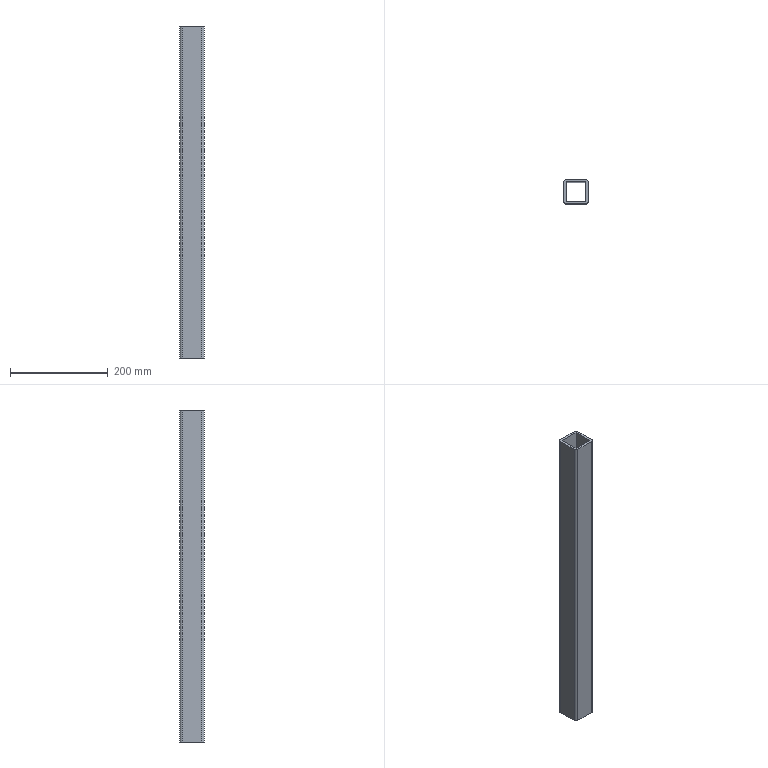Part | STEP file | SOLID | 1 solid | 14 faces | box 50 x 50 x 680 mm | volume 597407 mm3 | plane 10 | cylinder 4 | commonest cylinder face diameters 10 x4
STEP:
#1=CARTESIAN_POINT('',(0.,0.,0.));
#2=DIRECTION('',(0.,0.,1.));
#3=DIRECTION('',(1.,0.,0.));
#4=AXIS2_PLACEMENT_3D('',#1,#2,#3);
#5=CARTESIAN_POINT('',(-758.5,-310.,-70.));
#6=VERTEX_POINT('',#5);
#7=CARTESIAN_POINT('',(-758.5,-270.,-70.));
#8=VERTEX_POINT('',#7);
#9=CARTESIAN_POINT('',(-758.5,-310.,-70.));
#10=DIRECTION('',(0.,1.,0.));
#11=VECTOR('',#10,1.);
#12=LINE('',#9,#11);
#13=CARTESIAN_POINT('',(-758.5,-310.,-670.));
#14=DIRECTION('',(1.,0.,0.));
#15=DIRECTION('',(0.,1.,0.));
#16=AXIS2_PLACEMENT_3D('',#13,#14,#15);
#17=PLANE('',#16);
#18=CARTESIAN_POINT('',(0.,600.));
#19=DIRECTION('',(1.,0.));
#20=VECTOR('',#19,1.);
#21=LINE('',#18,#20);
#22=(GEOMETRIC_REPRESENTATION_CONTEXT(2)PARAMETRIC_REPRESENTATION_CONTEXT()REPRESENTATION_CONTEXT('',''));
#23=DEFINITIONAL_REPRESENTATION('',(#21),#22);
#24=PCURVE('',#17,#23);
#25=CARTESIAN_POINT('',(826.5,-310.,-70.));
#26=DIRECTION('',(0.,0.,1.));
#27=DIRECTION('',(0.,-1.,0.));
#28=AXIS2_PLACEMENT_3D('',#25,#26,#27);
#29=PLANE('',#28);
#30=CARTESIAN_POINT('',(0.,-1585.));
#31=DIRECTION('',(-1.,0.));
#32=VECTOR('',#31,1.);
#33=LINE('',#30,#32);
#34=(GEOMETRIC_REPRESENTATION_CONTEXT(2)PARAMETRIC_REPRESENTATION_CONTEXT()REPRESENTATION_CONTEXT('',''));
#35=DEFINITIONAL_REPRESENTATION('',(#33),#34);
#36=PCURVE('',#29,#35);
#37=SURFACE_CURVE('',#12,(#24,#36),.PCURVE_S1.);
#38=EDGE_CURVE('',#6,#8,#37,.T.);
#39=ORIENTED_EDGE('',*,*,#38,.T.);
#40=CARTESIAN_POINT('',(-758.5,-270.,-750.));
#41=VERTEX_POINT('',#40);
#42=CARTESIAN_POINT('',(-758.5,-270.,-670.));
#43=DIRECTION('',(0.,0.,1.));
#44=VECTOR('',#43,1.);
#45=LINE('',#42,#44);
#46=CARTESIAN_POINT('',(40.,0.));
#47=DIRECTION('',(0.,1.));
#48=VECTOR('',#47,1.);
#49=LINE('',#46,#48);
#50=(GEOMETRIC_REPRESENTATION_CONTEXT(2)PARAMETRIC_REPRESENTATION_CONTEXT()REPRESENTATION_CONTEXT('',''));
#51=DEFINITIONAL_REPRESENTATION('',(#49),#50);
#52=PCURVE('',#17,#51);
#53=CARTESIAN_POINT('',(-758.5,-270.,-670.));
#54=DIRECTION('',(0.,1.,0.));
#55=DIRECTION('',(-1.,0.,0.));
#56=AXIS2_PLACEMENT_3D('',#53,#54,#55);
#57=PLANE('',#56);
#58=CARTESIAN_POINT('',(0.,0.));
#59=DIRECTION('',(0.,1.));
#60=VECTOR('',#59,1.);
#61=LINE('',#58,#60);
#62=(GEOMETRIC_REPRESENTATION_CONTEXT(2)PARAMETRIC_REPRESENTATION_CONTEXT()REPRESENTATION_CONTEXT('',''));
#63=DEFINITIONAL_REPRESENTATION('',(#61),#62);
#64=PCURVE('',#57,#63);
#65=SURFACE_CURVE('',#45,(#52,#64),.PCURVE_S1.);
#66=EDGE_CURVE('',#41,#8,#65,.T.);
#67=ORIENTED_EDGE('',*,*,#66,.F.);
#68=CARTESIAN_POINT('',(-758.5,-310.,-750.));
#69=VERTEX_POINT('',#68);
#70=CARTESIAN_POINT('',(-758.5,-310.,-750.));
#71=DIRECTION('',(0.,1.,0.));
#72=VECTOR('',#71,1.);
#73=LINE('',#70,#72);
#74=CARTESIAN_POINT('',(0.,-80.));
#75=DIRECTION('',(1.,0.));
#76=VECTOR('',#75,1.);
#77=LINE('',#74,#76);
#78=(GEOMETRIC_REPRESENTATION_CONTEXT(2)PARAMETRIC_REPRESENTATION_CONTEXT()REPRESENTATION_CONTEXT('',''));
#79=DEFINITIONAL_REPRESENTATION('',(#77),#78);
#80=PCURVE('',#17,#79);
#81=CARTESIAN_POINT('',(796.5,-310.,-750.));
#82=DIRECTION('',(0.,0.,1.));
#83=DIRECTION('',(0.,-1.,0.));
#84=AXIS2_PLACEMENT_3D('',#81,#82,#83);
#85=PLANE('',#84);
#86=CARTESIAN_POINT('',(0.,-1555.));
#87=DIRECTION('',(-1.,0.));
#88=VECTOR('',#87,1.);
#89=LINE('',#86,#88);
#90=(GEOMETRIC_REPRESENTATION_CONTEXT(2)PARAMETRIC_REPRESENTATION_CONTEXT()REPRESENTATION_CONTEXT('',''));
#91=DEFINITIONAL_REPRESENTATION('',(#89),#90);
#92=PCURVE('',#85,#91);
#93=SURFACE_CURVE('',#73,(#80,#92),.PCURVE_S1.);
#94=EDGE_CURVE('',#69,#41,#93,.T.);
#95=ORIENTED_EDGE('',*,*,#94,.F.);
#96=CARTESIAN_POINT('',(-758.5,-310.,-670.));
#97=DIRECTION('',(0.,0.,1.));
#98=VECTOR('',#97,1.);
#99=LINE('',#96,#98);
#100=CARTESIAN_POINT('',(0.,0.));
#101=DIRECTION('',(0.,1.));
#102=VECTOR('',#101,1.);
#103=LINE('',#100,#102);
#104=(GEOMETRIC_REPRESENTATION_CONTEXT(2)PARAMETRIC_REPRESENTATION_CONTEXT()REPRESENTATION_CONTEXT('',''));
#105=DEFINITIONAL_REPRESENTATION('',(#103),#104);
#106=PCURVE('',#17,#105);
#107=CARTESIAN_POINT('',(-798.5,-310.,-670.));
#108=DIRECTION('',(0.,-1.,0.));
#109=DIRECTION('',(0.,0.,1.));
#110=AXIS2_PLACEMENT_3D('',#107,#108,#109);
#111=PLANE('',#110);
#112=CARTESIAN_POINT('',(0.,-40.));
#113=DIRECTION('',(1.,0.));
#114=VECTOR('',#113,1.);
#115=LINE('',#112,#114);
#116=(GEOMETRIC_REPRESENTATION_CONTEXT(2)PARAMETRIC_REPRESENTATION_CONTEXT()REPRESENTATION_CONTEXT('',''));
#117=DEFINITIONAL_REPRESENTATION('',(#115),#116);
#118=PCURVE('',#111,#117);
#119=SURFACE_CURVE('',#99,(#106,#118),.PCURVE_S1.);
#120=EDGE_CURVE('',#69,#6,#119,.T.);
#121=ORIENTED_EDGE('',*,*,#120,.T.);
#122=EDGE_LOOP('',(#39,#67,#95,#121));
#123=FACE_BOUND('',#122,.T.);
#124=ADVANCED_FACE('',(#123),#17,.F.);
#125=CARTESIAN_POINT('',(-798.5,-270.,-70.));
#126=VERTEX_POINT('',#125);
#127=CARTESIAN_POINT('',(-758.5,-270.,-70.));
#128=DIRECTION('',(-1.,0.,0.));
#129=VECTOR('',#128,1.);
#130=LINE('',#127,#129);
#131=CARTESIAN_POINT('',(0.,600.));
#132=DIRECTION('',(1.,0.));
#133=VECTOR('',#132,1.);
#134=LINE('',#131,#133);
#135=(GEOMETRIC_REPRESENTATION_CONTEXT(2)PARAMETRIC_REPRESENTATION_CONTEXT()REPRESENTATION_CONTEXT('',''));
#136=DEFINITIONAL_REPRESENTATION('',(#134),#135);
#137=PCURVE('',#57,#136);
#138=CARTESIAN_POINT('',(-40.,-1585.));
#139=DIRECTION('',(0.,-1.));
#140=VECTOR('',#139,1.);
#141=LINE('',#138,#140);
#142=(GEOMETRIC_REPRESENTATION_CONTEXT(2)PARAMETRIC_REPRESENTATION_CONTEXT()REPRESENTATION_CONTEXT('',''));
#143=DEFINITIONAL_REPRESENTATION('',(#141),#142);
#144=PCURVE('',#29,#143);
#145=SURFACE_CURVE('',#130,(#137,#144),.PCURVE_S1.);
#146=EDGE_CURVE('',#8,#126,#145,.T.);
#147=ORIENTED_EDGE('',*,*,#146,.T.);
#148=CARTESIAN_POINT('',(-798.5,-270.,-750.));
#149=VERTEX_POINT('',#148);
#150=CARTESIAN_POINT('',(-798.5,-270.,-670.));
#151=DIRECTION('',(0.,0.,1.));
#152=VECTOR('',#151,1.);
#153=LINE('',#150,#152);
#154=CARTESIAN_POINT('',(40.,0.));
#155=DIRECTION('',(0.,1.));
#156=VECTOR('',#155,1.);
#157=LINE('',#154,#156);
#158=(GEOMETRIC_REPRESENTATION_CONTEXT(2)PARAMETRIC_REPRESENTATION_CONTEXT()REPRESENTATION_CONTEXT('',''));
#159=DEFINITIONAL_REPRESENTATION('',(#157),#158);
#160=PCURVE('',#57,#159);
#161=CARTESIAN_POINT('',(-798.5,-270.,-670.));
#162=DIRECTION('',(-1.,0.,0.));
#163=DIRECTION('',(0.,0.,-1.));
#164=AXIS2_PLACEMENT_3D('',#161,#162,#163);
#165=PLANE('',#164);
#166=CARTESIAN_POINT('',(0.,0.));
#167=DIRECTION('',(-1.,0.));
#168=VECTOR('',#167,1.);
#169=LINE('',#166,#168);
#170=(GEOMETRIC_REPRESENTATION_CONTEXT(2)PARAMETRIC_REPRESENTATION_CONTEXT()REPRESENTATION_CONTEXT('',''));
#171=DEFINITIONAL_REPRESENTATION('',(#169),#170);
#172=PCURVE('',#165,#171);
#173=SURFACE_CURVE('',#153,(#160,#172),.PCURVE_S1.);
#174=EDGE_CURVE('',#149,#126,#173,.T.);
#175=ORIENTED_EDGE('',*,*,#174,.F.);
#176=CARTESIAN_POINT('',(-758.5,-270.,-750.));
#177=DIRECTION('',(-1.,0.,0.));
#178=VECTOR('',#177,1.);
#179=LINE('',#176,#178);
#180=CARTESIAN_POINT('',(0.,-80.));
#181=DIRECTION('',(1.,0.));
#182=VECTOR('',#181,1.);
#183=LINE('',#180,#182);
#184=(GEOMETRIC_REPRESENTATION_CONTEXT(2)PARAMETRIC_REPRESENTATION_CONTEXT()REPRESENTATION_CONTEXT('',''));
#185=DEFINITIONAL_REPRESENTATION('',(#183),#184);
#186=PCURVE('',#57,#185);
#187=CARTESIAN_POINT('',(-40.,-1555.));
#188=DIRECTION('',(0.,-1.));
#189=VECTOR('',#188,1.);
#190=LINE('',#187,#189);
#191=(GEOMETRIC_REPRESENTATION_CONTEXT(2)PARAMETRIC_REPRESENTATION_CONTEXT()REPRESENTATION_CONTEXT('',''));
#192=DEFINITIONAL_REPRESENTATION('',(#190),#191);
#193=PCURVE('',#85,#192);
#194=SURFACE_CURVE('',#179,(#186,#193),.PCURVE_S1.);
#195=EDGE_CURVE('',#41,#149,#194,.T.);
#196=ORIENTED_EDGE('',*,*,#195,.F.);
#197=ORIENTED_EDGE('',*,*,#66,.T.);
#198=EDGE_LOOP('',(#147,#175,#196,#197));
#199=FACE_BOUND('',#198,.T.);
#200=ADVANCED_FACE('',(#199),#57,.F.);
#201=CARTESIAN_POINT('',(-798.5,-310.,-70.));
#202=VERTEX_POINT('',#201);
#203=CARTESIAN_POINT('',(-798.5,-270.,-70.));
#204=DIRECTION('',(0.,-1.,0.));
#205=VECTOR('',#204,1.);
#206=LINE('',#203,#205);
#207=CARTESIAN_POINT('',(-600.,0.));
#208=DIRECTION('',(0.,1.));
#209=VECTOR('',#208,1.);
#210=LINE('',#207,#209);
#211=(GEOMETRIC_REPRESENTATION_CONTEXT(2)PARAMETRIC_REPRESENTATION_CONTEXT()REPRESENTATION_CONTEXT('',''));
#212=DEFINITIONAL_REPRESENTATION('',(#210),#211);
#213=PCURVE('',#165,#212);
#214=CARTESIAN_POINT('',(-40.,-1625.));
#215=DIRECTION('',(1.,0.));
#216=VECTOR('',#215,1.);
#217=LINE('',#214,#216);
#218=(GEOMETRIC_REPRESENTATION_CONTEXT(2)PARAMETRIC_REPRESENTATION_CONTEXT()REPRESENTATION_CONTEXT('',''));
#219=DEFINITIONAL_REPRESENTATION('',(#217),#218);
#220=PCURVE('',#29,#219);
#221=SURFACE_CURVE('',#206,(#213,#220),.PCURVE_S1.);
#222=EDGE_CURVE('',#126,#202,#221,.T.);
#223=ORIENTED_EDGE('',*,*,#222,.T.);
#224=CARTESIAN_POINT('',(-798.5,-310.,-750.));
#225=VERTEX_POINT('',#224);
#226=CARTESIAN_POINT('',(-798.5,-310.,-670.));
#227=DIRECTION('',(0.,0.,1.));
#228=VECTOR('',#227,1.);
#229=LINE('',#226,#228);
#230=CARTESIAN_POINT('',(0.,40.));
#231=DIRECTION('',(-1.,0.));
#232=VECTOR('',#231,1.);
#233=LINE('',#230,#232);
#234=(GEOMETRIC_REPRESENTATION_CONTEXT(2)PARAMETRIC_REPRESENTATION_CONTEXT()REPRESENTATION_CONTEXT('',''));
#235=DEFINITIONAL_REPRESENTATION('',(#233),#234);
#236=PCURVE('',#165,#235);
#237=CARTESIAN_POINT('',(0.,0.));
#238=DIRECTION('',(1.,0.));
#239=VECTOR('',#238,1.);
#240=LINE('',#237,#239);
#241=(GEOMETRIC_REPRESENTATION_CONTEXT(2)PARAMETRIC_REPRESENTATION_CONTEXT()REPRESENTATION_CONTEXT('',''));
#242=DEFINITIONAL_REPRESENTATION('',(#240),#241);
#243=PCURVE('',#111,#242);
#244=SURFACE_CURVE('',#229,(#236,#243),.PCURVE_S1.);
#245=EDGE_CURVE('',#225,#202,#244,.T.);
#246=ORIENTED_EDGE('',*,*,#245,.F.);
#247=CARTESIAN_POINT('',(-798.5,-270.,-750.));
#248=DIRECTION('',(0.,-1.,0.));
#249=VECTOR('',#248,1.);
#250=LINE('',#247,#249);
#251=CARTESIAN_POINT('',(80.,0.));
#252=DIRECTION('',(0.,1.));
#253=VECTOR('',#252,1.);
#254=LINE('',#251,#253);
#255=(GEOMETRIC_REPRESENTATION_CONTEXT(2)PARAMETRIC_REPRESENTATION_CONTEXT()REPRESENTATION_CONTEXT('',''));
#256=DEFINITIONAL_REPRESENTATION('',(#254),#255);
#257=PCURVE('',#165,#256);
#258=CARTESIAN_POINT('',(-40.,-1595.));
#259=DIRECTION('',(1.,0.));
#260=VECTOR('',#259,1.);
#261=LINE('',#258,#260);
#262=(GEOMETRIC_REPRESENTATION_CONTEXT(2)PARAMETRIC_REPRESENTATION_CONTEXT()REPRESENTATION_CONTEXT('',''));
#263=DEFINITIONAL_REPRESENTATION('',(#261),#262);
#264=PCURVE('',#85,#263);
#265=SURFACE_CURVE('',#250,(#257,#264),.PCURVE_S1.);
#266=EDGE_CURVE('',#149,#225,#265,.T.);
#267=ORIENTED_EDGE('',*,*,#266,.F.);
#268=ORIENTED_EDGE('',*,*,#174,.T.);
#269=EDGE_LOOP('',(#223,#246,#267,#268));
#270=FACE_BOUND('',#269,.T.);
#271=ADVANCED_FACE('',(#270),#165,.F.);
#272=CARTESIAN_POINT('',(-753.5,-270.,-70.));
#273=VERTEX_POINT('',#272);
#274=CARTESIAN_POINT('',(-753.5,-310.,-70.));
#275=VERTEX_POINT('',#274);
#276=CARTESIAN_POINT('',(-753.5,-270.,-70.));
#277=DIRECTION('',(0.,-1.,0.));
#278=VECTOR('',#277,1.);
#279=LINE('',#276,#278);
#280=CARTESIAN_POINT('',(-753.5,-270.,-670.));
#281=DIRECTION('',(-1.,0.,0.));
#282=DIRECTION('',(0.,-1.,0.));
#283=AXIS2_PLACEMENT_3D('',#280,#281,#282);
#284=PLANE('',#283);
#285=CARTESIAN_POINT('',(0.,600.));
#286=DIRECTION('',(1.,0.));
#287=VECTOR('',#286,1.);
#288=LINE('',#285,#287);
#289=(GEOMETRIC_REPRESENTATION_CONTEXT(2)PARAMETRIC_REPRESENTATION_CONTEXT()REPRESENTATION_CONTEXT('',''));
#290=DEFINITIONAL_REPRESENTATION('',(#288),#289);
#291=PCURVE('',#284,#290);
#292=CARTESIAN_POINT('',(-40.,-1580.));
#293=DIRECTION('',(1.,0.));
#294=VECTOR('',#293,1.);
#295=LINE('',#292,#294);
#296=(GEOMETRIC_REPRESENTATION_CONTEXT(2)PARAMETRIC_REPRESENTATION_CONTEXT()REPRESENTATION_CONTEXT('',''));
#297=DEFINITIONAL_REPRESENTATION('',(#295),#296);
#298=PCURVE('',#29,#297);
#299=SURFACE_CURVE('',#279,(#291,#298),.PCURVE_S1.);
#300=EDGE_CURVE('',#273,#275,#299,.T.);
#301=ORIENTED_EDGE('',*,*,#300,.T.);
#302=CARTESIAN_POINT('',(-753.5,-310.,-750.));
#303=VERTEX_POINT('',#302);
#304=CARTESIAN_POINT('',(-753.5,-310.,-670.));
#305=DIRECTION('',(0.,0.,1.));
#306=VECTOR('',#305,1.);
#307=LINE('',#304,#306);
#308=CARTESIAN_POINT('',(40.,0.));
#309=DIRECTION('',(0.,1.));
#310=VECTOR('',#309,1.);
#311=LINE('',#308,#310);
#312=(GEOMETRIC_REPRESENTATION_CONTEXT(2)PARAMETRIC_REPRESENTATION_CONTEXT()REPRESENTATION_CONTEXT('',''));
#313=DEFINITIONAL_REPRESENTATION('',(#311),#312);
#314=PCURVE('',#284,#313);
#315=CARTESIAN_POINT('',(-758.5,-310.,-670.));
#316=DIRECTION('',(0.,0.,1.));
#317=DIRECTION('',(0.,1.,0.));
#318=AXIS2_PLACEMENT_3D('',#315,#316,#317);
#319=CYLINDRICAL_SURFACE('',#318,5.);
#320=CARTESIAN_POINT('',(4.712,0.));
#321=DIRECTION('',(0.,1.));
#322=VECTOR('',#321,1.);
#323=LINE('',#320,#322);
#324=(GEOMETRIC_REPRESENTATION_CONTEXT(2)PARAMETRIC_REPRESENTATION_CONTEXT()REPRESENTATION_CONTEXT('',''));
#325=DEFINITIONAL_REPRESENTATION('',(#323),#324);
#326=PCURVE('',#319,#325);
#327=SURFACE_CURVE('',#307,(#314,#326),.PCURVE_S1.);
#328=EDGE_CURVE('',#303,#275,#327,.T.);
#329=ORIENTED_EDGE('',*,*,#328,.F.);
#330=CARTESIAN_POINT('',(-753.5,-270.,-750.));
#331=VERTEX_POINT('',#330);
#332=CARTESIAN_POINT('',(-753.5,-270.,-750.));
#333=DIRECTION('',(0.,-1.,0.));
#334=VECTOR('',#333,1.);
#335=LINE('',#332,#334);
#336=CARTESIAN_POINT('',(0.,-80.));
#337=DIRECTION('',(1.,0.));
#338=VECTOR('',#337,1.);
#339=LINE('',#336,#338);
#340=(GEOMETRIC_REPRESENTATION_CONTEXT(2)PARAMETRIC_REPRESENTATION_CONTEXT()REPRESENTATION_CONTEXT('',''));
#341=DEFINITIONAL_REPRESENTATION('',(#339),#340);
#342=PCURVE('',#284,#341);
#343=CARTESIAN_POINT('',(-40.,-1550.));
#344=DIRECTION('',(1.,0.));
#345=VECTOR('',#344,1.);
#346=LINE('',#343,#345);
#347=(GEOMETRIC_REPRESENTATION_CONTEXT(2)PARAMETRIC_REPRESENTATION_CONTEXT()REPRESENTATION_CONTEXT('',''));
#348=DEFINITIONAL_REPRESENTATION('',(#346),#347);
#349=PCURVE('',#85,#348);
#350=SURFACE_CURVE('',#335,(#342,#349),.PCURVE_S1.);
#351=EDGE_CURVE('',#331,#303,#350,.T.);
#352=ORIENTED_EDGE('',*,*,#351,.F.);
#353=CARTESIAN_POINT('',(-753.5,-270.,-670.));
#354=DIRECTION('',(0.,0.,1.));
#355=VECTOR('',#354,1.);
#356=LINE('',#353,#355);
#357=CARTESIAN_POINT('',(0.,0.));
#358=DIRECTION('',(0.,1.));
#359=VECTOR('',#358,1.);
#360=LINE('',#357,#359);
#361=(GEOMETRIC_REPRESENTATION_CONTEXT(2)PARAMETRIC_REPRESENTATION_CONTEXT()REPRESENTATION_CONTEXT('',''));
#362=DEFINITIONAL_REPRESENTATION('',(#360),#361);
#363=PCURVE('',#284,#362);
#364=CARTESIAN_POINT('',(-758.5,-270.,-670.));
#365=DIRECTION('',(0.,0.,1.));
#366=DIRECTION('',(0.,1.,0.));
#367=AXIS2_PLACEMENT_3D('',#364,#365,#366);
#368=CYLINDRICAL_SURFACE('',#367,5.);
#369=CARTESIAN_POINT('',(4.712,0.));
#370=DIRECTION('',(0.,1.));
#371=VECTOR('',#370,1.);
#372=LINE('',#369,#371);
#373=(GEOMETRIC_REPRESENTATION_CONTEXT(2)PARAMETRIC_REPRESENTATION_CONTEXT()REPRESENTATION_CONTEXT('',''));
#374=DEFINITIONAL_REPRESENTATION('',(#372),#373);
#375=PCURVE('',#368,#374);
#376=SURFACE_CURVE('',#356,(#363,#375),.PCURVE_S1.);
#377=EDGE_CURVE('',#331,#273,#376,.T.);
#378=ORIENTED_EDGE('',*,*,#377,.T.);
#379=EDGE_LOOP('',(#301,#329,#352,#378));
#380=FACE_BOUND('',#379,.T.);
#381=ADVANCED_FACE('',(#380),#284,.F.);
#382=CARTESIAN_POINT('',(-758.5,-315.,-70.));
#383=VERTEX_POINT('',#382);
#384=CARTESIAN_POINT('',(-758.5,-310.,-70.));
#385=DIRECTION('',(0.,0.,-1.));
#386=DIRECTION('',(0.,1.,0.));
#387=AXIS2_PLACEMENT_3D('',#384,#385,#386);
#388=CIRCLE('',#387,5.);
#389=CARTESIAN_POINT('',(6.283,600.));
#390=DIRECTION('',(-1.,0.));
#391=VECTOR('',#390,1.);
#392=LINE('',#389,#391);
#393=(GEOMETRIC_REPRESENTATION_CONTEXT(2)PARAMETRIC_REPRESENTATION_CONTEXT()REPRESENTATION_CONTEXT('',''));
#394=DEFINITIONAL_REPRESENTATION('',(#392),#393);
#395=PCURVE('',#319,#394);
#396=CARTESIAN_POINT('',(-5.,-1585.));
#397=CARTESIAN_POINT('',(-5.,-1576.34));
#398=CARTESIAN_POINT('',(2.5,-1580.67));
#399=CARTESIAN_POINT('',(10.,-1585.));
#400=CARTESIAN_POINT('',(2.5,-1589.33));
#401=CARTESIAN_POINT('',(-5.,-1593.66));
#402=CARTESIAN_POINT('',(-5.,-1585.));
#403=(BOUNDED_CURVE()B_SPLINE_CURVE(2,(#396,#397,#398,#399,#400,#401,#402),.UNSPECIFIED.,.T.,.F.)B_SPLINE_CURVE_WITH_KNOTS((1,2,2,2,2,1),(-2.094,0.,2.094,4.189,6.283,8.378),.UNSPECIFIED.)CURVE()GEOMETRIC_REPRESENTATION_ITEM()RATIONAL_B_SPLINE_CURVE((1.,0.5,1.,0.5,1.,0.5,1.))REPRESENTATION_ITEM(''));
#404=(GEOMETRIC_REPRESENTATION_CONTEXT(2)PARAMETRIC_REPRESENTATION_CONTEXT()REPRESENTATION_CONTEXT('',''));
#405=DEFINITIONAL_REPRESENTATION('',(#403),#404);
#406=PCURVE('',#29,#405);
#407=SURFACE_CURVE('',#388,(#395,#406),.PCURVE_S1.);
#408=EDGE_CURVE('',#275,#383,#407,.T.);
#409=ORIENTED_EDGE('',*,*,#408,.T.);
#410=CARTESIAN_POINT('',(-758.5,-315.,-750.));
#411=VERTEX_POINT('',#410);
#412=CARTESIAN_POINT('',(-758.5,-315.,-670.));
#413=DIRECTION('',(0.,0.,1.));
#414=VECTOR('',#413,1.);
#415=LINE('',#412,#414);
#416=CARTESIAN_POINT('',(3.142,0.));
#417=DIRECTION('',(0.,1.));
#418=VECTOR('',#417,1.);
#419=LINE('',#416,#418);
#420=(GEOMETRIC_REPRESENTATION_CONTEXT(2)PARAMETRIC_REPRESENTATION_CONTEXT()REPRESENTATION_CONTEXT('',''));
#421=DEFINITIONAL_REPRESENTATION('',(#419),#420);
#422=PCURVE('',#319,#421);
#423=CARTESIAN_POINT('',(-758.5,-315.,-670.));
#424=DIRECTION('',(0.,1.,0.));
#425=DIRECTION('',(0.,0.,-1.));
#426=AXIS2_PLACEMENT_3D('',#423,#424,#425);
#427=PLANE('',#426);
#428=CARTESIAN_POINT('',(0.,0.));
#429=DIRECTION('',(-1.,0.));
#430=VECTOR('',#429,1.);
#431=LINE('',#428,#430);
#432=(GEOMETRIC_REPRESENTATION_CONTEXT(2)PARAMETRIC_REPRESENTATION_CONTEXT()REPRESENTATION_CONTEXT('',''));
#433=DEFINITIONAL_REPRESENTATION('',(#431),#432);
#434=PCURVE('',#427,#433);
#435=SURFACE_CURVE('',#415,(#422,#434),.PCURVE_S1.);
#436=EDGE_CURVE('',#411,#383,#435,.T.);
#437=ORIENTED_EDGE('',*,*,#436,.F.);
#438=CARTESIAN_POINT('',(-758.5,-310.,-750.));
#439=DIRECTION('',(0.,0.,-1.));
#440=DIRECTION('',(0.,-1.,0.));
#441=AXIS2_PLACEMENT_3D('',#438,#439,#440);
#442=CIRCLE('',#441,5.);
#443=CARTESIAN_POINT('',(9.425,-80.));
#444=DIRECTION('',(-1.,0.));
#445=VECTOR('',#444,1.);
#446=LINE('',#443,#445);
#447=(GEOMETRIC_REPRESENTATION_CONTEXT(2)PARAMETRIC_REPRESENTATION_CONTEXT()REPRESENTATION_CONTEXT('',''));
#448=DEFINITIONAL_REPRESENTATION('',(#446),#447);
#449=PCURVE('',#319,#448);
#450=CARTESIAN_POINT('',(5.,-1555.));
#451=CARTESIAN_POINT('',(5.,-1563.66));
#452=CARTESIAN_POINT('',(-2.5,-1559.33));
#453=CARTESIAN_POINT('',(-10.,-1555.));
#454=CARTESIAN_POINT('',(-2.5,-1550.67));
#455=CARTESIAN_POINT('',(5.,-1546.34));
#456=CARTESIAN_POINT('',(5.,-1555.));
#457=(BOUNDED_CURVE()B_SPLINE_CURVE(2,(#450,#451,#452,#453,#454,#455,#456),.UNSPECIFIED.,.T.,.F.)B_SPLINE_CURVE_WITH_KNOTS((1,2,2,2,2,1),(-2.094,0.,2.094,4.189,6.283,8.378),.UNSPECIFIED.)CURVE()GEOMETRIC_REPRESENTATION_ITEM()RATIONAL_B_SPLINE_CURVE((1.,0.5,1.,0.5,1.,0.5,1.))REPRESENTATION_ITEM(''));
#458=(GEOMETRIC_REPRESENTATION_CONTEXT(2)PARAMETRIC_REPRESENTATION_CONTEXT()REPRESENTATION_CONTEXT('',''));
#459=DEFINITIONAL_REPRESENTATION('',(#457),#458);
#460=PCURVE('',#85,#459);
#461=SURFACE_CURVE('',#442,(#449,#460),.PCURVE_S1.);
#462=EDGE_CURVE('',#303,#411,#461,.T.);
#463=ORIENTED_EDGE('',*,*,#462,.F.);
#464=ORIENTED_EDGE('',*,*,#328,.T.);
#465=EDGE_LOOP('',(#409,#437,#463,#464));
#466=FACE_BOUND('',#465,.T.);
#467=ADVANCED_FACE('',(#466),#319,.T.);
#468=CARTESIAN_POINT('',(-798.5,-315.,-70.));
#469=VERTEX_POINT('',#468);
#470=CARTESIAN_POINT('',(-758.5,-315.,-70.));
#471=DIRECTION('',(-1.,0.,0.));
#472=VECTOR('',#471,1.);
#473=LINE('',#470,#472);
#474=CARTESIAN_POINT('',(-600.,0.));
#475=DIRECTION('',(0.,1.));
#476=VECTOR('',#475,1.);
#477=LINE('',#474,#476);
#478=(GEOMETRIC_REPRESENTATION_CONTEXT(2)PARAMETRIC_REPRESENTATION_CONTEXT()REPRESENTATION_CONTEXT('',''));
#479=DEFINITIONAL_REPRESENTATION('',(#477),#478);
#480=PCURVE('',#427,#479);
#481=CARTESIAN_POINT('',(5.,-1585.));
#482=DIRECTION('',(0.,-1.));
#483=VECTOR('',#482,1.);
#484=LINE('',#481,#483);
#485=(GEOMETRIC_REPRESENTATION_CONTEXT(2)PARAMETRIC_REPRESENTATION_CONTEXT()REPRESENTATION_CONTEXT('',''));
#486=DEFINITIONAL_REPRESENTATION('',(#484),#485);
#487=PCURVE('',#29,#486);
#488=SURFACE_CURVE('',#473,(#480,#487),.PCURVE_S1.);
#489=EDGE_CURVE('',#383,#469,#488,.T.);
#490=ORIENTED_EDGE('',*,*,#489,.T.);
#491=CARTESIAN_POINT('',(-798.5,-315.,-750.));
#492=VERTEX_POINT('',#491);
#493=CARTESIAN_POINT('',(-798.5,-315.,-670.));
#494=DIRECTION('',(0.,0.,1.));
#495=VECTOR('',#494,1.);
#496=LINE('',#493,#495);
#497=CARTESIAN_POINT('',(0.,40.));
#498=DIRECTION('',(-1.,0.));
#499=VECTOR('',#498,1.);
#500=LINE('',#497,#499);
#501=(GEOMETRIC_REPRESENTATION_CONTEXT(2)PARAMETRIC_REPRESENTATION_CONTEXT()REPRESENTATION_CONTEXT('',''));
#502=DEFINITIONAL_REPRESENTATION('',(#500),#501);
#503=PCURVE('',#427,#502);
#504=CARTESIAN_POINT('',(-798.5,-310.,-670.));
#505=DIRECTION('',(0.,0.,1.));
#506=DIRECTION('',(0.,1.,0.));
#507=AXIS2_PLACEMENT_3D('',#504,#505,#506);
#508=CYLINDRICAL_SURFACE('',#507,5.);
#509=CARTESIAN_POINT('',(3.142,0.));
#510=DIRECTION('',(0.,1.));
#511=VECTOR('',#510,1.);
#512=LINE('',#509,#511);
#513=(GEOMETRIC_REPRESENTATION_CONTEXT(2)PARAMETRIC_REPRESENTATION_CONTEXT()REPRESENTATION_CONTEXT('',''));
#514=DEFINITIONAL_REPRESENTATION('',(#512),#513);
#515=PCURVE('',#508,#514);
#516=SURFACE_CURVE('',#496,(#503,#515),.PCURVE_S1.);
#517=EDGE_CURVE('',#492,#469,#516,.T.);
#518=ORIENTED_EDGE('',*,*,#517,.F.);
#519=CARTESIAN_POINT('',(-758.5,-315.,-750.));
#520=DIRECTION('',(-1.,0.,0.));
#521=VECTOR('',#520,1.);
#522=LINE('',#519,#521);
#523=CARTESIAN_POINT('',(80.,0.));
#524=DIRECTION('',(0.,1.));
#525=VECTOR('',#524,1.);
#526=LINE('',#523,#525);
#527=(GEOMETRIC_REPRESENTATION_CONTEXT(2)PARAMETRIC_REPRESENTATION_CONTEXT()REPRESENTATION_CONTEXT('',''));
#528=DEFINITIONAL_REPRESENTATION('',(#526),#527);
#529=PCURVE('',#427,#528);
#530=CARTESIAN_POINT('',(5.,-1555.));
#531=DIRECTION('',(0.,-1.));
#532=VECTOR('',#531,1.);
#533=LINE('',#530,#532);
#534=(GEOMETRIC_REPRESENTATION_CONTEXT(2)PARAMETRIC_REPRESENTATION_CONTEXT()REPRESENTATION_CONTEXT('',''));
#535=DEFINITIONAL_REPRESENTATION('',(#533),#534);
#536=PCURVE('',#85,#535);
#537=SURFACE_CURVE('',#522,(#529,#536),.PCURVE_S1.);
#538=EDGE_CURVE('',#411,#492,#537,.T.);
#539=ORIENTED_EDGE('',*,*,#538,.F.);
#540=ORIENTED_EDGE('',*,*,#436,.T.);
#541=EDGE_LOOP('',(#490,#518,#539,#540));
#542=FACE_BOUND('',#541,.T.);
#543=ADVANCED_FACE('',(#542),#427,.F.);
#544=CARTESIAN_POINT('',(-803.5,-310.,-70.));
#545=VERTEX_POINT('',#544);
#546=CARTESIAN_POINT('',(-798.5,-310.,-70.));
#547=DIRECTION('',(0.,0.,-1.));
#548=DIRECTION('',(0.,1.,0.));
#549=AXIS2_PLACEMENT_3D('',#546,#547,#548);
#550=CIRCLE('',#549,5.);
#551=CARTESIAN_POINT('',(6.283,600.));
#552=DIRECTION('',(-1.,0.));
#553=VECTOR('',#552,1.);
#554=LINE('',#551,#553);
#555=(GEOMETRIC_REPRESENTATION_CONTEXT(2)PARAMETRIC_REPRESENTATION_CONTEXT()REPRESENTATION_CONTEXT('',''));
#556=DEFINITIONAL_REPRESENTATION('',(#554),#555);
#557=PCURVE('',#508,#556);
#558=CARTESIAN_POINT('',(-5.,-1625.));
#559=CARTESIAN_POINT('',(-5.,-1616.34));
#560=CARTESIAN_POINT('',(2.5,-1620.67));
#561=CARTESIAN_POINT('',(10.,-1625.));
#562=CARTESIAN_POINT('',(2.5,-1629.33));
#563=CARTESIAN_POINT('',(-5.,-1633.66));
#564=CARTESIAN_POINT('',(-5.,-1625.));
#565=(BOUNDED_CURVE()B_SPLINE_CURVE(2,(#558,#559,#560,#561,#562,#563,#564),.UNSPECIFIED.,.T.,.F.)B_SPLINE_CURVE_WITH_KNOTS((1,2,2,2,2,1),(-2.094,0.,2.094,4.189,6.283,8.378),.UNSPECIFIED.)CURVE()GEOMETRIC_REPRESENTATION_ITEM()RATIONAL_B_SPLINE_CURVE((1.,0.5,1.,0.5,1.,0.5,1.))REPRESENTATION_ITEM(''));
#566=(GEOMETRIC_REPRESENTATION_CONTEXT(2)PARAMETRIC_REPRESENTATION_CONTEXT()REPRESENTATION_CONTEXT('',''));
#567=DEFINITIONAL_REPRESENTATION('',(#565),#566);
#568=PCURVE('',#29,#567);
#569=SURFACE_CURVE('',#550,(#557,#568),.PCURVE_S1.);
#570=EDGE_CURVE('',#469,#545,#569,.T.);
#571=ORIENTED_EDGE('',*,*,#570,.T.);
#572=CARTESIAN_POINT('',(-803.5,-310.,-750.));
#573=VERTEX_POINT('',#572);
#574=CARTESIAN_POINT('',(-803.5,-310.,-670.));
#575=DIRECTION('',(0.,0.,1.));
#576=VECTOR('',#575,1.);
#577=LINE('',#574,#576);
#578=CARTESIAN_POINT('',(1.571,0.));
#579=DIRECTION('',(0.,1.));
#580=VECTOR('',#579,1.);
#581=LINE('',#578,#580);
#582=(GEOMETRIC_REPRESENTATION_CONTEXT(2)PARAMETRIC_REPRESENTATION_CONTEXT()REPRESENTATION_CONTEXT('',''));
#583=DEFINITIONAL_REPRESENTATION('',(#581),#582);
#584=PCURVE('',#508,#583);
#585=CARTESIAN_POINT('',(-803.5,-310.,-670.));
#586=DIRECTION('',(1.,0.,0.));
#587=DIRECTION('',(0.,0.,1.));
#588=AXIS2_PLACEMENT_3D('',#585,#586,#587);
#589=PLANE('',#588);
#590=CARTESIAN_POINT('',(0.,0.));
#591=DIRECTION('',(1.,0.));
#592=VECTOR('',#591,1.);
#593=LINE('',#590,#592);
#594=(GEOMETRIC_REPRESENTATION_CONTEXT(2)PARAMETRIC_REPRESENTATION_CONTEXT()REPRESENTATION_CONTEXT('',''));
#595=DEFINITIONAL_REPRESENTATION('',(#593),#594);
#596=PCURVE('',#589,#595);
#597=SURFACE_CURVE('',#577,(#584,#596),.PCURVE_S1.);
#598=EDGE_CURVE('',#573,#545,#597,.T.);
#599=ORIENTED_EDGE('',*,*,#598,.F.);
#600=CARTESIAN_POINT('',(-798.5,-310.,-750.));
#601=DIRECTION('',(0.,0.,-1.));
#602=DIRECTION('',(0.,-1.,0.));
#603=AXIS2_PLACEMENT_3D('',#600,#601,#602);
#604=CIRCLE('',#603,5.);
#605=CARTESIAN_POINT('',(3.142,-80.));
#606=DIRECTION('',(-1.,0.));
#607=VECTOR('',#606,1.);
#608=LINE('',#605,#607);
#609=(GEOMETRIC_REPRESENTATION_CONTEXT(2)PARAMETRIC_REPRESENTATION_CONTEXT()REPRESENTATION_CONTEXT('',''));
#610=DEFINITIONAL_REPRESENTATION('',(#608),#609);
#611=PCURVE('',#508,#610);
#612=CARTESIAN_POINT('',(5.,-1595.));
#613=CARTESIAN_POINT('',(5.,-1603.66));
#614=CARTESIAN_POINT('',(-2.5,-1599.33));
#615=CARTESIAN_POINT('',(-10.,-1595.));
#616=CARTESIAN_POINT('',(-2.5,-1590.67));
#617=CARTESIAN_POINT('',(5.,-1586.34));
#618=CARTESIAN_POINT('',(5.,-1595.));
#619=(BOUNDED_CURVE()B_SPLINE_CURVE(2,(#612,#613,#614,#615,#616,#617,#618),.UNSPECIFIED.,.T.,.F.)B_SPLINE_CURVE_WITH_KNOTS((1,2,2,2,2,1),(-2.094,0.,2.094,4.189,6.283,8.378),.UNSPECIFIED.)CURVE()GEOMETRIC_REPRESENTATION_ITEM()RATIONAL_B_SPLINE_CURVE((1.,0.5,1.,0.5,1.,0.5,1.))REPRESENTATION_ITEM(''));
#620=(GEOMETRIC_REPRESENTATION_CONTEXT(2)PARAMETRIC_REPRESENTATION_CONTEXT()REPRESENTATION_CONTEXT('',''));
#621=DEFINITIONAL_REPRESENTATION('',(#619),#620);
#622=PCURVE('',#85,#621);
#623=SURFACE_CURVE('',#604,(#611,#622),.PCURVE_S1.);
#624=EDGE_CURVE('',#492,#573,#623,.T.);
#625=ORIENTED_EDGE('',*,*,#624,.F.);
#626=ORIENTED_EDGE('',*,*,#517,.T.);
#627=EDGE_LOOP('',(#571,#599,#625,#626));
#628=FACE_BOUND('',#627,.T.);
#629=ADVANCED_FACE('',(#628),#508,.T.);
#630=CARTESIAN_POINT('',(-803.5,-270.,-70.));
#631=VERTEX_POINT('',#630);
#632=CARTESIAN_POINT('',(-803.5,-310.,-70.));
#633=DIRECTION('',(0.,1.,0.));
#634=VECTOR('',#633,1.);
#635=LINE('',#632,#634);
#636=CARTESIAN_POINT('',(600.,0.));
#637=DIRECTION('',(0.,-1.));
#638=VECTOR('',#637,1.);
#639=LINE('',#636,#638);
#640=(GEOMETRIC_REPRESENTATION_CONTEXT(2)PARAMETRIC_REPRESENTATION_CONTEXT()REPRESENTATION_CONTEXT('',''));
#641=DEFINITIONAL_REPRESENTATION('',(#639),#640);
#642=PCURVE('',#589,#641);
#643=CARTESIAN_POINT('',(0.,-1630.));
#644=DIRECTION('',(-1.,0.));
#645=VECTOR('',#644,1.);
#646=LINE('',#643,#645);
#647=(GEOMETRIC_REPRESENTATION_CONTEXT(2)PARAMETRIC_REPRESENTATION_CONTEXT()REPRESENTATION_CONTEXT('',''));
#648=DEFINITIONAL_REPRESENTATION('',(#646),#647);
#649=PCURVE('',#29,#648);
#650=SURFACE_CURVE('',#635,(#642,#649),.PCURVE_S1.);
#651=EDGE_CURVE('',#545,#631,#650,.T.);
#652=ORIENTED_EDGE('',*,*,#651,.T.);
#653=CARTESIAN_POINT('',(-803.5,-270.,-750.));
#654=VERTEX_POINT('',#653);
#655=CARTESIAN_POINT('',(-803.5,-270.,-670.));
#656=DIRECTION('',(0.,0.,1.));
#657=VECTOR('',#656,1.);
#658=LINE('',#655,#657);
#659=CARTESIAN_POINT('',(0.,-40.));
#660=DIRECTION('',(1.,0.));
#661=VECTOR('',#660,1.);
#662=LINE('',#659,#661);
#663=(GEOMETRIC_REPRESENTATION_CONTEXT(2)PARAMETRIC_REPRESENTATION_CONTEXT()REPRESENTATION_CONTEXT('',''));
#664=DEFINITIONAL_REPRESENTATION('',(#662),#663);
#665=PCURVE('',#589,#664);
#666=CARTESIAN_POINT('',(-798.5,-270.,-670.));
#667=DIRECTION('',(0.,0.,1.));
#668=DIRECTION('',(0.,1.,0.));
#669=AXIS2_PLACEMENT_3D('',#666,#667,#668);
#670=CYLINDRICAL_SURFACE('',#669,5.);
#671=CARTESIAN_POINT('',(1.571,0.));
#672=DIRECTION('',(0.,1.));
#673=VECTOR('',#672,1.);
#674=LINE('',#671,#673);
#675=(GEOMETRIC_REPRESENTATION_CONTEXT(2)PARAMETRIC_REPRESENTATION_CONTEXT()REPRESENTATION_CONTEXT('',''));
#676=DEFINITIONAL_REPRESENTATION('',(#674),#675);
#677=PCURVE('',#670,#676);
#678=SURFACE_CURVE('',#658,(#665,#677),.PCURVE_S1.);
#679=EDGE_CURVE('',#654,#631,#678,.T.);
#680=ORIENTED_EDGE('',*,*,#679,.F.);
#681=CARTESIAN_POINT('',(-803.5,-310.,-750.));
#682=DIRECTION('',(0.,1.,0.));
#683=VECTOR('',#682,1.);
#684=LINE('',#681,#683);
#685=CARTESIAN_POINT('',(-80.,0.));
#686=DIRECTION('',(0.,-1.));
#687=VECTOR('',#686,1.);
#688=LINE('',#685,#687);
#689=(GEOMETRIC_REPRESENTATION_CONTEXT(2)PARAMETRIC_REPRESENTATION_CONTEXT()REPRESENTATION_CONTEXT('',''));
#690=DEFINITIONAL_REPRESENTATION('',(#688),#689);
#691=PCURVE('',#589,#690);
#692=CARTESIAN_POINT('',(0.,-1600.));
#693=DIRECTION('',(-1.,0.));
#694=VECTOR('',#693,1.);
#695=LINE('',#692,#694);
#696=(GEOMETRIC_REPRESENTATION_CONTEXT(2)PARAMETRIC_REPRESENTATION_CONTEXT()REPRESENTATION_CONTEXT('',''));
#697=DEFINITIONAL_REPRESENTATION('',(#695),#696);
#698=PCURVE('',#85,#697);
#699=SURFACE_CURVE('',#684,(#691,#698),.PCURVE_S1.);
#700=EDGE_CURVE('',#573,#654,#699,.T.);
#701=ORIENTED_EDGE('',*,*,#700,.F.);
#702=ORIENTED_EDGE('',*,*,#598,.T.);
#703=EDGE_LOOP('',(#652,#680,#701,#702));
#704=FACE_BOUND('',#703,.T.);
#705=ADVANCED_FACE('',(#704),#589,.F.);
#706=CARTESIAN_POINT('',(-798.5,-265.,-70.));
#707=VERTEX_POINT('',#706);
#708=CARTESIAN_POINT('',(-798.5,-270.,-70.));
#709=DIRECTION('',(0.,0.,-1.));
#710=DIRECTION('',(0.,1.,0.));
#711=AXIS2_PLACEMENT_3D('',#708,#709,#710);
#712=CIRCLE('',#711,5.);
#713=CARTESIAN_POINT('',(6.283,600.));
#714=DIRECTION('',(-1.,0.));
#715=VECTOR('',#714,1.);
#716=LINE('',#713,#715);
#717=(GEOMETRIC_REPRESENTATION_CONTEXT(2)PARAMETRIC_REPRESENTATION_CONTEXT()REPRESENTATION_CONTEXT('',''));
#718=DEFINITIONAL_REPRESENTATION('',(#716),#717);
#719=PCURVE('',#670,#718);
#720=CARTESIAN_POINT('',(-45.,-1625.));
#721=CARTESIAN_POINT('',(-45.,-1616.34));
#722=CARTESIAN_POINT('',(-37.5,-1620.67));
#723=CARTESIAN_POINT('',(-30.,-1625.));
#724=CARTESIAN_POINT('',(-37.5,-1629.33));
#725=CARTESIAN_POINT('',(-45.,-1633.66));
#726=CARTESIAN_POINT('',(-45.,-1625.));
#727=(BOUNDED_CURVE()B_SPLINE_CURVE(2,(#720,#721,#722,#723,#724,#725,#726),.UNSPECIFIED.,.T.,.F.)B_SPLINE_CURVE_WITH_KNOTS((1,2,2,2,2,1),(-2.094,0.,2.094,4.189,6.283,8.378),.UNSPECIFIED.)CURVE()GEOMETRIC_REPRESENTATION_ITEM()RATIONAL_B_SPLINE_CURVE((1.,0.5,1.,0.5,1.,0.5,1.))REPRESENTATION_ITEM(''));
#728=(GEOMETRIC_REPRESENTATION_CONTEXT(2)PARAMETRIC_REPRESENTATION_CONTEXT()REPRESENTATION_CONTEXT('',''));
#729=DEFINITIONAL_REPRESENTATION('',(#727),#728);
#730=PCURVE('',#29,#729);
#731=SURFACE_CURVE('',#712,(#719,#730),.PCURVE_S1.);
#732=EDGE_CURVE('',#631,#707,#731,.T.);
#733=ORIENTED_EDGE('',*,*,#732,.T.);
#734=CARTESIAN_POINT('',(-798.5,-265.,-750.));
#735=VERTEX_POINT('',#734);
#736=CARTESIAN_POINT('',(-798.5,-265.,-670.));
#737=DIRECTION('',(0.,0.,1.));
#738=VECTOR('',#737,1.);
#739=LINE('',#736,#738);
#740=CARTESIAN_POINT('',(0.,0.));
#741=DIRECTION('',(0.,1.));
#742=VECTOR('',#741,1.);
#743=LINE('',#740,#742);
#744=(GEOMETRIC_REPRESENTATION_CONTEXT(2)PARAMETRIC_REPRESENTATION_CONTEXT()REPRESENTATION_CONTEXT('',''));
#745=DEFINITIONAL_REPRESENTATION('',(#743),#744);
#746=PCURVE('',#670,#745);
#747=CARTESIAN_POINT('',(-798.5,-265.,-670.));
#748=DIRECTION('',(0.,-1.,0.));
#749=DIRECTION('',(1.,0.,0.));
#750=AXIS2_PLACEMENT_3D('',#747,#748,#749);
#751=PLANE('',#750);
#752=CARTESIAN_POINT('',(0.,0.));
#753=DIRECTION('',(0.,1.));
#754=VECTOR('',#753,1.);
#755=LINE('',#752,#754);
#756=(GEOMETRIC_REPRESENTATION_CONTEXT(2)PARAMETRIC_REPRESENTATION_CONTEXT()REPRESENTATION_CONTEXT('',''));
#757=DEFINITIONAL_REPRESENTATION('',(#755),#756);
#758=PCURVE('',#751,#757);
#759=SURFACE_CURVE('',#739,(#746,#758),.PCURVE_S1.);
#760=EDGE_CURVE('',#735,#707,#759,.T.);
#761=ORIENTED_EDGE('',*,*,#760,.F.);
#762=CARTESIAN_POINT('',(-798.5,-270.,-750.));
#763=DIRECTION('',(0.,0.,-1.));
#764=DIRECTION('',(0.,-1.,0.));
#765=AXIS2_PLACEMENT_3D('',#762,#763,#764);
#766=CIRCLE('',#765,5.);
#767=CARTESIAN_POINT('',(3.142,-80.));
#768=DIRECTION('',(-1.,0.));
#769=VECTOR('',#768,1.);
#770=LINE('',#767,#769);
#771=(GEOMETRIC_REPRESENTATION_CONTEXT(2)PARAMETRIC_REPRESENTATION_CONTEXT()REPRESENTATION_CONTEXT('',''));
#772=DEFINITIONAL_REPRESENTATION('',(#770),#771);
#773=PCURVE('',#670,#772);
#774=CARTESIAN_POINT('',(-35.,-1595.));
#775=CARTESIAN_POINT('',(-35.,-1603.66));
#776=CARTESIAN_POINT('',(-42.5,-1599.33));
#777=CARTESIAN_POINT('',(-50.,-1595.));
#778=CARTESIAN_POINT('',(-42.5,-1590.67));
#779=CARTESIAN_POINT('',(-35.,-1586.34));
#780=CARTESIAN_POINT('',(-35.,-1595.));
#781=(BOUNDED_CURVE()B_SPLINE_CURVE(2,(#774,#775,#776,#777,#778,#779,#780),.UNSPECIFIED.,.T.,.F.)B_SPLINE_CURVE_WITH_KNOTS((1,2,2,2,2,1),(-2.094,0.,2.094,4.189,6.283,8.378),.UNSPECIFIED.)CURVE()GEOMETRIC_REPRESENTATION_ITEM()RATIONAL_B_SPLINE_CURVE((1.,0.5,1.,0.5,1.,0.5,1.))REPRESENTATION_ITEM(''));
#782=(GEOMETRIC_REPRESENTATION_CONTEXT(2)PARAMETRIC_REPRESENTATION_CONTEXT()REPRESENTATION_CONTEXT('',''));
#783=DEFINITIONAL_REPRESENTATION('',(#781),#782);
#784=PCURVE('',#85,#783);
#785=SURFACE_CURVE('',#766,(#773,#784),.PCURVE_S1.);
#786=EDGE_CURVE('',#654,#735,#785,.T.);
#787=ORIENTED_EDGE('',*,*,#786,.F.);
#788=ORIENTED_EDGE('',*,*,#679,.T.);
#789=EDGE_LOOP('',(#733,#761,#787,#788));
#790=FACE_BOUND('',#789,.T.);
#791=ADVANCED_FACE('',(#790),#670,.T.);
#792=CARTESIAN_POINT('',(-758.5,-265.,-70.));
#793=VERTEX_POINT('',#792);
#794=CARTESIAN_POINT('',(-798.5,-265.,-70.));
#795=DIRECTION('',(1.,0.,0.));
#796=VECTOR('',#795,1.);
#797=LINE('',#794,#796);
#798=CARTESIAN_POINT('',(0.,600.));
#799=DIRECTION('',(1.,0.));
#800=VECTOR('',#799,1.);
#801=LINE('',#798,#800);
#802=(GEOMETRIC_REPRESENTATION_CONTEXT(2)PARAMETRIC_REPRESENTATION_CONTEXT()REPRESENTATION_CONTEXT('',''));
#803=DEFINITIONAL_REPRESENTATION('',(#801),#802);
#804=PCURVE('',#751,#803);
#805=CARTESIAN_POINT('',(-45.,-1625.));
#806=DIRECTION('',(0.,1.));
#807=VECTOR('',#806,1.);
#808=LINE('',#805,#807);
#809=(GEOMETRIC_REPRESENTATION_CONTEXT(2)PARAMETRIC_REPRESENTATION_CONTEXT()REPRESENTATION_CONTEXT('',''));
#810=DEFINITIONAL_REPRESENTATION('',(#808),#809);
#811=PCURVE('',#29,#810);
#812=SURFACE_CURVE('',#797,(#804,#811),.PCURVE_S1.);
#813=EDGE_CURVE('',#707,#793,#812,.T.);
#814=ORIENTED_EDGE('',*,*,#813,.T.);
#815=CARTESIAN_POINT('',(-758.5,-265.,-750.));
#816=VERTEX_POINT('',#815);
#817=CARTESIAN_POINT('',(-758.5,-265.,-670.));
#818=DIRECTION('',(0.,0.,1.));
#819=VECTOR('',#818,1.);
#820=LINE('',#817,#819);
#821=CARTESIAN_POINT('',(40.,0.));
#822=DIRECTION('',(0.,1.));
#823=VECTOR('',#822,1.);
#824=LINE('',#821,#823);
#825=(GEOMETRIC_REPRESENTATION_CONTEXT(2)PARAMETRIC_REPRESENTATION_CONTEXT()REPRESENTATION_CONTEXT('',''));
#826=DEFINITIONAL_REPRESENTATION('',(#824),#825);
#827=PCURVE('',#751,#826);
#828=CARTESIAN_POINT('',(6.283,0.));
#829=DIRECTION('',(0.,1.));
#830=VECTOR('',#829,1.);
#831=LINE('',#828,#830);
#832=(GEOMETRIC_REPRESENTATION_CONTEXT(2)PARAMETRIC_REPRESENTATION_CONTEXT()REPRESENTATION_CONTEXT('',''));
#833=DEFINITIONAL_REPRESENTATION('',(#831),#832);
#834=PCURVE('',#368,#833);
#835=SURFACE_CURVE('',#820,(#827,#834),.PCURVE_S1.);
#836=EDGE_CURVE('',#816,#793,#835,.T.);
#837=ORIENTED_EDGE('',*,*,#836,.F.);
#838=CARTESIAN_POINT('',(-798.5,-265.,-750.));
#839=DIRECTION('',(1.,0.,0.));
#840=VECTOR('',#839,1.);
#841=LINE('',#838,#840);
#842=CARTESIAN_POINT('',(0.,-80.));
#843=DIRECTION('',(1.,0.));
#844=VECTOR('',#843,1.);
#845=LINE('',#842,#844);
#846=(GEOMETRIC_REPRESENTATION_CONTEXT(2)PARAMETRIC_REPRESENTATION_CONTEXT()REPRESENTATION_CONTEXT('',''));
#847=DEFINITIONAL_REPRESENTATION('',(#845),#846);
#848=PCURVE('',#751,#847);
#849=CARTESIAN_POINT('',(-45.,-1595.));
#850=DIRECTION('',(0.,1.));
#851=VECTOR('',#850,1.);
#852=LINE('',#849,#851);
#853=(GEOMETRIC_REPRESENTATION_CONTEXT(2)PARAMETRIC_REPRESENTATION_CONTEXT()REPRESENTATION_CONTEXT('',''));
#854=DEFINITIONAL_REPRESENTATION('',(#852),#853);
#855=PCURVE('',#85,#854);
#856=SURFACE_CURVE('',#841,(#848,#855),.PCURVE_S1.);
#857=EDGE_CURVE('',#735,#816,#856,.T.);
#858=ORIENTED_EDGE('',*,*,#857,.F.);
#859=ORIENTED_EDGE('',*,*,#760,.T.);
#860=EDGE_LOOP('',(#814,#837,#858,#859));
#861=FACE_BOUND('',#860,.T.);
#862=ADVANCED_FACE('',(#861),#751,.F.);
#863=CARTESIAN_POINT('',(-758.5,-270.,-70.));
#864=DIRECTION('',(0.,0.,-1.));
#865=DIRECTION('',(0.,1.,0.));
#866=AXIS2_PLACEMENT_3D('',#863,#864,#865);
#867=CIRCLE('',#866,5.);
#868=CARTESIAN_POINT('',(6.283,600.));
#869=DIRECTION('',(-1.,0.));
#870=VECTOR('',#869,1.);
#871=LINE('',#868,#870);
#872=(GEOMETRIC_REPRESENTATION_CONTEXT(2)PARAMETRIC_REPRESENTATION_CONTEXT()REPRESENTATION_CONTEXT('',''));
#873=DEFINITIONAL_REPRESENTATION('',(#871),#872);
#874=PCURVE('',#368,#873);
#875=CARTESIAN_POINT('',(-45.,-1585.));
#876=CARTESIAN_POINT('',(-45.,-1576.34));
#877=CARTESIAN_POINT('',(-37.5,-1580.67));
#878=CARTESIAN_POINT('',(-30.,-1585.));
#879=CARTESIAN_POINT('',(-37.5,-1589.33));
#880=CARTESIAN_POINT('',(-45.,-1593.66));
#881=CARTESIAN_POINT('',(-45.,-1585.));
#882=(BOUNDED_CURVE()B_SPLINE_CURVE(2,(#875,#876,#877,#878,#879,#880,#881),.UNSPECIFIED.,.T.,.F.)B_SPLINE_CURVE_WITH_KNOTS((1,2,2,2,2,1),(-2.094,0.,2.094,4.189,6.283,8.378),.UNSPECIFIED.)CURVE()GEOMETRIC_REPRESENTATION_ITEM()RATIONAL_B_SPLINE_CURVE((1.,0.5,1.,0.5,1.,0.5,1.))REPRESENTATION_ITEM(''));
#883=(GEOMETRIC_REPRESENTATION_CONTEXT(2)PARAMETRIC_REPRESENTATION_CONTEXT()REPRESENTATION_CONTEXT('',''));
#884=DEFINITIONAL_REPRESENTATION('',(#882),#883);
#885=PCURVE('',#29,#884);
#886=SURFACE_CURVE('',#867,(#874,#885),.PCURVE_S1.);
#887=EDGE_CURVE('',#793,#273,#886,.T.);
#888=ORIENTED_EDGE('',*,*,#887,.T.);
#889=ORIENTED_EDGE('',*,*,#377,.F.);
#890=CARTESIAN_POINT('',(-758.5,-270.,-750.));
#891=DIRECTION('',(0.,0.,-1.));
#892=DIRECTION('',(0.,-1.,0.));
#893=AXIS2_PLACEMENT_3D('',#890,#891,#892);
#894=CIRCLE('',#893,5.);
#895=CARTESIAN_POINT('',(9.425,-80.));
#896=DIRECTION('',(-1.,0.));
#897=VECTOR('',#896,1.);
#898=LINE('',#895,#897);
#899=(GEOMETRIC_REPRESENTATION_CONTEXT(2)PARAMETRIC_REPRESENTATION_CONTEXT()REPRESENTATION_CONTEXT('',''));
#900=DEFINITIONAL_REPRESENTATION('',(#898),#899);
#901=PCURVE('',#368,#900);
#902=CARTESIAN_POINT('',(-35.,-1555.));
#903=CARTESIAN_POINT('',(-35.,-1563.66));
#904=CARTESIAN_POINT('',(-42.5,-1559.33));
#905=CARTESIAN_POINT('',(-50.,-1555.));
#906=CARTESIAN_POINT('',(-42.5,-1550.67));
#907=CARTESIAN_POINT('',(-35.,-1546.34));
#908=CARTESIAN_POINT('',(-35.,-1555.));
#909=(BOUNDED_CURVE()B_SPLINE_CURVE(2,(#902,#903,#904,#905,#906,#907,#908),.UNSPECIFIED.,.T.,.F.)B_SPLINE_CURVE_WITH_KNOTS((1,2,2,2,2,1),(-2.094,0.,2.094,4.189,6.283,8.378),.UNSPECIFIED.)CURVE()GEOMETRIC_REPRESENTATION_ITEM()RATIONAL_B_SPLINE_CURVE((1.,0.5,1.,0.5,1.,0.5,1.))REPRESENTATION_ITEM(''));
#910=(GEOMETRIC_REPRESENTATION_CONTEXT(2)PARAMETRIC_REPRESENTATION_CONTEXT()REPRESENTATION_CONTEXT('',''));
#911=DEFINITIONAL_REPRESENTATION('',(#909),#910);
#912=PCURVE('',#85,#911);
#913=SURFACE_CURVE('',#894,(#901,#912),.PCURVE_S1.);
#914=EDGE_CURVE('',#816,#331,#913,.T.);
#915=ORIENTED_EDGE('',*,*,#914,.F.);
#916=ORIENTED_EDGE('',*,*,#836,.T.);
#917=EDGE_LOOP('',(#888,#889,#915,#916));
#918=FACE_BOUND('',#917,.T.);
#919=ADVANCED_FACE('',(#918),#368,.T.);
#920=CARTESIAN_POINT('',(-798.5,-310.,-70.));
#921=DIRECTION('',(1.,0.,0.));
#922=VECTOR('',#921,1.);
#923=LINE('',#920,#922);
#924=CARTESIAN_POINT('',(600.,0.));
#925=DIRECTION('',(0.,-1.));
#926=VECTOR('',#925,1.);
#927=LINE('',#924,#926);
#928=(GEOMETRIC_REPRESENTATION_CONTEXT(2)PARAMETRIC_REPRESENTATION_CONTEXT()REPRESENTATION_CONTEXT('',''));
#929=DEFINITIONAL_REPRESENTATION('',(#927),#928);
#930=PCURVE('',#111,#929);
#931=CARTESIAN_POINT('',(0.,-1625.));
#932=DIRECTION('',(0.,1.));
#933=VECTOR('',#932,1.);
#934=LINE('',#931,#933);
#935=(GEOMETRIC_REPRESENTATION_CONTEXT(2)PARAMETRIC_REPRESENTATION_CONTEXT()REPRESENTATION_CONTEXT('',''));
#936=DEFINITIONAL_REPRESENTATION('',(#934),#935);
#937=PCURVE('',#29,#936);
#938=SURFACE_CURVE('',#923,(#930,#937),.PCURVE_S1.);
#939=EDGE_CURVE('',#202,#6,#938,.T.);
#940=ORIENTED_EDGE('',*,*,#939,.T.);
#941=ORIENTED_EDGE('',*,*,#120,.F.);
#942=CARTESIAN_POINT('',(-798.5,-310.,-750.));
#943=DIRECTION('',(1.,0.,0.));
#944=VECTOR('',#943,1.);
#945=LINE('',#942,#944);
#946=CARTESIAN_POINT('',(-80.,0.));
#947=DIRECTION('',(0.,-1.));
#948=VECTOR('',#947,1.);
#949=LINE('',#946,#948);
#950=(GEOMETRIC_REPRESENTATION_CONTEXT(2)PARAMETRIC_REPRESENTATION_CONTEXT()REPRESENTATION_CONTEXT('',''));
#951=DEFINITIONAL_REPRESENTATION('',(#949),#950);
#952=PCURVE('',#111,#951);
#953=CARTESIAN_POINT('',(0.,-1595.));
#954=DIRECTION('',(0.,1.));
#955=VECTOR('',#954,1.);
#956=LINE('',#953,#955);
#957=(GEOMETRIC_REPRESENTATION_CONTEXT(2)PARAMETRIC_REPRESENTATION_CONTEXT()REPRESENTATION_CONTEXT('',''));
#958=DEFINITIONAL_REPRESENTATION('',(#956),#957);
#959=PCURVE('',#85,#958);
#960=SURFACE_CURVE('',#945,(#952,#959),.PCURVE_S1.);
#961=EDGE_CURVE('',#225,#69,#960,.T.);
#962=ORIENTED_EDGE('',*,*,#961,.F.);
#963=ORIENTED_EDGE('',*,*,#245,.T.);
#964=EDGE_LOOP('',(#940,#941,#962,#963));
#965=FACE_BOUND('',#964,.T.);
#966=ADVANCED_FACE('',(#965),#111,.F.);
#967=ORIENTED_EDGE('',*,*,#351,.T.);
#968=ORIENTED_EDGE('',*,*,#462,.T.);
#969=ORIENTED_EDGE('',*,*,#538,.T.);
#970=ORIENTED_EDGE('',*,*,#624,.T.);
#971=ORIENTED_EDGE('',*,*,#700,.T.);
#972=ORIENTED_EDGE('',*,*,#786,.T.);
#973=ORIENTED_EDGE('',*,*,#857,.T.);
#974=ORIENTED_EDGE('',*,*,#914,.T.);
#975=EDGE_LOOP('',(#967,#968,#969,#970,#971,#972,#973,#974));
#976=FACE_BOUND('',#975,.T.);
#977=ORIENTED_EDGE('',*,*,#94,.T.);
#978=ORIENTED_EDGE('',*,*,#195,.T.);
#979=ORIENTED_EDGE('',*,*,#266,.T.);
#980=ORIENTED_EDGE('',*,*,#961,.T.);
#981=EDGE_LOOP('',(#977,#978,#979,#980));
#982=FACE_BOUND('',#981,.T.);
#983=ADVANCED_FACE('',(#976,#982),#85,.F.);
#984=ORIENTED_EDGE('',*,*,#300,.F.);
#985=ORIENTED_EDGE('',*,*,#887,.F.);
#986=ORIENTED_EDGE('',*,*,#813,.F.);
#987=ORIENTED_EDGE('',*,*,#732,.F.);
#988=ORIENTED_EDGE('',*,*,#651,.F.);
#989=ORIENTED_EDGE('',*,*,#570,.F.);
#990=ORIENTED_EDGE('',*,*,#489,.F.);
#991=ORIENTED_EDGE('',*,*,#408,.F.);
#992=EDGE_LOOP('',(#984,#985,#986,#987,#988,#989,#990,#991));
#993=FACE_BOUND('',#992,.T.);
#994=ORIENTED_EDGE('',*,*,#38,.F.);
#995=ORIENTED_EDGE('',*,*,#939,.F.);
#996=ORIENTED_EDGE('',*,*,#222,.F.);
#997=ORIENTED_EDGE('',*,*,#146,.F.);
#998=EDGE_LOOP('',(#994,#995,#996,#997));
#999=FACE_BOUND('',#998,.T.);
#1000=ADVANCED_FACE('',(#993,#999),#29,.T.);
#1001=CLOSED_SHELL('',(#124,#200,#271,#381,#467,#543,#629,#705,#791,#862,#919,#966,#983,#1000));
#1002=MANIFOLD_SOLID_BREP('',#1001);
#1003=(LENGTH_UNIT()NAMED_UNIT(*)SI_UNIT(.MILLI.,.METRE.));
#1004=UNCERTAINTY_MEASURE_WITH_UNIT(LENGTH_MEASURE(0.0000001),#1003,'','');
#1005=(NAMED_UNIT(*)PLANE_ANGLE_UNIT()SI_UNIT($,.RADIAN.));
#1006=(NAMED_UNIT(*)SI_UNIT($,.STERADIAN.)SOLID_ANGLE_UNIT());
#1007=(GEOMETRIC_REPRESENTATION_CONTEXT(3)GLOBAL_UNCERTAINTY_ASSIGNED_CONTEXT((#1004))GLOBAL_UNIT_ASSIGNED_CONTEXT((#1003,#1005,#1006))REPRESENTATION_CONTEXT('',''));
#1008=ADVANCED_BREP_SHAPE_REPRESENTATION('',(#4,#1002),#1007);